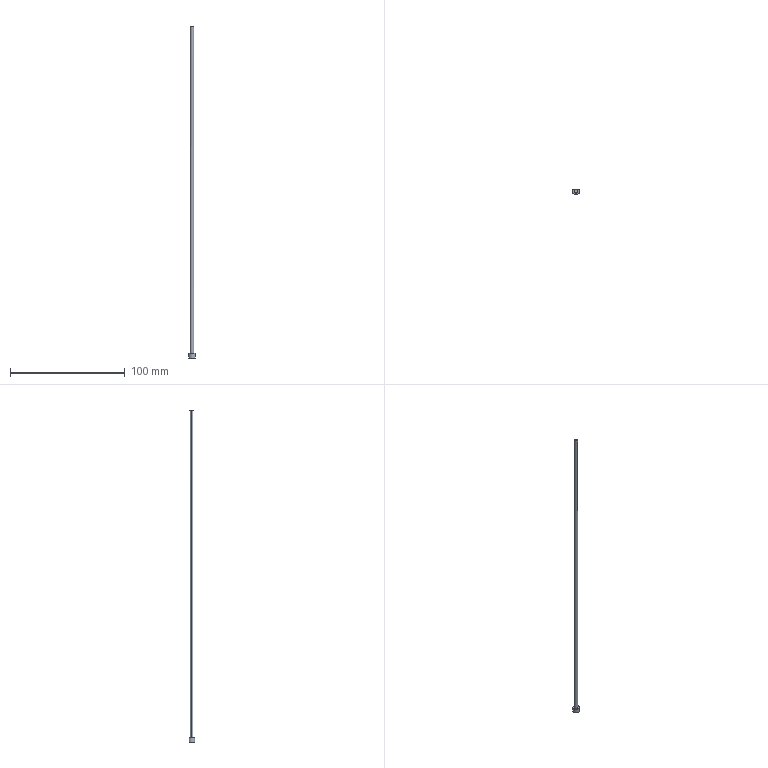Part | Creo | 1 solid | 7 faces | box 6 x 5 x 289.623 mm | volume 2118 mm3 | plane 4 | cylinder 3 | commonest cylinder face diameters 3 x2 6 x1
STEP:
#1=CARTESIAN_POINT('',(60.264,64.5,-292.));
#2=VERTEX_POINT('',#1);
#3=CARTESIAN_POINT('',(59.5,62.5,-292.));
#4=VERTEX_POINT('',#3);
#5=CARTESIAN_POINT('',(62.5,62.5,-292.));
#6=DIRECTION('',(0.,0.,1.));
#7=DIRECTION('',(-0.7454,0.6667,0.));
#8=AXIS2_PLACEMENT_3D('',#5,#6,#7);
#9=CIRCLE('',#8,3.);
#10=EDGE_CURVE('',#2,#4,#9,.T.);
#11=ORIENTED_EDGE('',*,*,#10,.F.);
#12=CARTESIAN_POINT('',(64.736,64.5,-292.));
#13=VERTEX_POINT('',#12);
#14=CARTESIAN_POINT('',(64.736,64.5,-292.));
#15=DIRECTION('',(-1.,0.,0.));
#16=VECTOR('',#15,4.472);
#17=LINE('',#14,#16);
#18=EDGE_CURVE('',#13,#2,#17,.T.);
#19=ORIENTED_EDGE('',*,*,#18,.F.);
#20=CARTESIAN_POINT('',(62.5,62.5,-292.));
#21=DIRECTION('',(0.,0.,1.));
#22=DIRECTION('',(-1.,0.,0.));
#23=AXIS2_PLACEMENT_3D('',#20,#21,#22);
#24=CIRCLE('',#23,3.);
#25=EDGE_CURVE('',#4,#13,#24,.T.);
#26=ORIENTED_EDGE('',*,*,#25,.F.);
#27=EDGE_LOOP('',(#11,#19,#26));
#28=FACE_OUTER_BOUND('',#27,.F.);
#29=CARTESIAN_POINT('',(64.,62.5,-292.));
#30=VERTEX_POINT('',#29);
#31=CARTESIAN_POINT('',(61.,62.5,-292.));
#32=VERTEX_POINT('',#31);
#33=CARTESIAN_POINT('',(62.5,62.5,-292.));
#34=DIRECTION('',(0.,0.,-1.));
#35=DIRECTION('',(1.,0.,0.));
#36=AXIS2_PLACEMENT_3D('',#33,#34,#35);
#37=CIRCLE('',#36,1.5);
#38=EDGE_CURVE('',#30,#32,#37,.T.);
#39=ORIENTED_EDGE('',*,*,#38,.F.);
#40=CARTESIAN_POINT('',(62.5,62.5,-292.));
#41=DIRECTION('',(0.,0.,-1.));
#42=DIRECTION('',(-1.,0.,0.));
#43=AXIS2_PLACEMENT_3D('',#40,#41,#42);
#44=CIRCLE('',#43,1.5);
#45=EDGE_CURVE('',#32,#30,#44,.T.);
#46=ORIENTED_EDGE('',*,*,#45,.F.);
#47=EDGE_LOOP('',(#39,#46));
#48=FACE_BOUND('',#47,.F.);
#49=CARTESIAN_POINT('',(62.5,62.5,-292.));
#50=DIRECTION('',(0.,0.,1.));
#51=DIRECTION('',(-1.,0.,0.));
#52=AXIS2_PLACEMENT_3D('',#49,#50,#51);
#53=PLANE('',#52);
#54=ADVANCED_FACE('',(#28,#48),#53,.T.);
#55=ORIENTED_EDGE('',*,*,#38,.T.);
#56=CARTESIAN_POINT('',(61.,62.5,-6.377));
#57=VERTEX_POINT('',#56);
#58=CARTESIAN_POINT('',(61.,62.5,-292.));
#59=DIRECTION('',(0.,0.000000001,1.));
#60=VECTOR('',#59,285.623);
#61=LINE('',#58,#60);
#62=EDGE_CURVE('',#32,#57,#61,.T.);
#63=ORIENTED_EDGE('',*,*,#62,.T.);
#64=CARTESIAN_POINT('',(64.,62.5,-6.535));
#65=VERTEX_POINT('',#64);
#66=CARTESIAN_POINT('',(61.,62.5,-6.377));
#67=CARTESIAN_POINT('',(61.,62.146,-6.377));
#68=CARTESIAN_POINT('',(61.223,61.523,-6.389));
#69=CARTESIAN_POINT('',(61.946,61.064,-6.427));
#70=CARTESIAN_POINT('',(62.5,60.968,-6.456));
#71=CARTESIAN_POINT('',(63.054,61.064,-6.485));
#72=CARTESIAN_POINT('',(63.777,61.523,-6.523));
#73=CARTESIAN_POINT('',(64.,62.146,-6.535));
#74=CARTESIAN_POINT('',(64.,62.5,-6.535));
#75=B_SPLINE_CURVE_WITH_KNOTS('',3,(#66,#67,#68,#69,#70,#71,#72,#73,#74),.UNSPECIFIED.,.F.,.F.,(4,1,1,1,1,1,4),(0.,0.25,0.375,0.5,0.625,0.75,1.),.UNSPECIFIED.);
#76=EDGE_CURVE('',#57,#65,#75,.T.);
#77=ORIENTED_EDGE('',*,*,#76,.T.);
#78=CARTESIAN_POINT('',(64.,62.5,-292.));
#79=DIRECTION('',(0.,0.,1.));
#80=VECTOR('',#79,285.465);
#81=LINE('',#78,#80);
#82=EDGE_CURVE('',#30,#65,#81,.T.);
#83=ORIENTED_EDGE('',*,*,#82,.F.);
#84=EDGE_LOOP('',(#55,#63,#77,#83));
#85=FACE_OUTER_BOUND('',#84,.F.);
#86=CARTESIAN_POINT('',(62.5,62.5,-352.221));
#87=DIRECTION('',(0.,0.,1.));
#88=DIRECTION('',(-1.,0.,0.));
#89=AXIS2_PLACEMENT_3D('',#86,#87,#88);
#90=CYLINDRICAL_SURFACE('',#89,1.5);
#91=ADVANCED_FACE('',(#85),#90,.T.);
#92=ORIENTED_EDGE('',*,*,#45,.T.);
#93=ORIENTED_EDGE('',*,*,#82,.T.);
#94=CARTESIAN_POINT('',(64.,62.5,-6.535));
#95=CARTESIAN_POINT('',(64.,62.854,-6.535));
#96=CARTESIAN_POINT('',(63.777,63.477,-6.523));
#97=CARTESIAN_POINT('',(63.054,63.936,-6.485));
#98=CARTESIAN_POINT('',(62.5,64.032,-6.456));
#99=CARTESIAN_POINT('',(61.946,63.936,-6.427));
#100=CARTESIAN_POINT('',(61.223,63.477,-6.389));
#101=CARTESIAN_POINT('',(61.,62.854,-6.377));
#102=CARTESIAN_POINT('',(61.,62.5,-6.377));
#103=B_SPLINE_CURVE_WITH_KNOTS('',3,(#94,#95,#96,#97,#98,#99,#100,#101,#102),.UNSPECIFIED.,.F.,.F.,(4,1,1,1,1,1,4),(0.,0.25,0.375,0.5,0.625,0.75,1.),.UNSPECIFIED.);
#104=EDGE_CURVE('',#65,#57,#103,.T.);
#105=ORIENTED_EDGE('',*,*,#104,.T.);
#106=ORIENTED_EDGE('',*,*,#62,.F.);
#107=EDGE_LOOP('',(#92,#93,#105,#106));
#108=FACE_OUTER_BOUND('',#107,.F.);
#109=CARTESIAN_POINT('',(62.5,62.5,-352.221));
#110=DIRECTION('',(0.,0.,1.));
#111=DIRECTION('',(-1.,0.,0.));
#112=AXIS2_PLACEMENT_3D('',#109,#110,#111);
#113=CYLINDRICAL_SURFACE('',#112,1.5);
#114=ADVANCED_FACE('',(#108),#113,.T.);
#115=ORIENTED_EDGE('',*,*,#76,.F.);
#116=ORIENTED_EDGE('',*,*,#104,.F.);
#117=EDGE_LOOP('',(#115,#116));
#118=FACE_OUTER_BOUND('',#117,.F.);
#119=CARTESIAN_POINT('',(308.361,-226.75,-19.338));
#120=DIRECTION('',(0.05232,-0.000000032,0.9986));
#121=DIRECTION('',(-0.000000001,-1.,-0.000000032));
#122=AXIS2_PLACEMENT_3D('',#119,#120,#121);
#123=PLANE('',#122);
#124=ADVANCED_FACE('',(#118),#123,.T.);
#125=CARTESIAN_POINT('',(60.264,64.5,-296.));
#126=VERTEX_POINT('',#125);
#127=CARTESIAN_POINT('',(60.264,64.5,-292.));
#128=DIRECTION('',(0.,0.,-1.));
#129=VECTOR('',#128,4.);
#130=LINE('',#127,#129);
#131=EDGE_CURVE('',#2,#126,#130,.T.);
#132=ORIENTED_EDGE('',*,*,#131,.F.);
#133=ORIENTED_EDGE('',*,*,#10,.T.);
#134=ORIENTED_EDGE('',*,*,#25,.T.);
#135=CARTESIAN_POINT('',(64.736,64.5,-296.));
#136=VERTEX_POINT('',#135);
#137=CARTESIAN_POINT('',(64.736,64.5,-296.));
#138=DIRECTION('',(0.,0.,1.));
#139=VECTOR('',#138,4.);
#140=LINE('',#137,#139);
#141=EDGE_CURVE('',#136,#13,#140,.T.);
#142=ORIENTED_EDGE('',*,*,#141,.F.);
#143=CARTESIAN_POINT('',(59.5,62.5,-296.));
#144=VERTEX_POINT('',#143);
#145=CARTESIAN_POINT('',(62.5,62.5,-296.));
#146=DIRECTION('',(0.,0.,-1.));
#147=DIRECTION('',(0.7454,0.6667,0.));
#148=AXIS2_PLACEMENT_3D('',#145,#146,#147);
#149=CIRCLE('',#148,3.);
#150=EDGE_CURVE('',#136,#144,#149,.T.);
#151=ORIENTED_EDGE('',*,*,#150,.T.);
#152=CARTESIAN_POINT('',(62.5,62.5,-296.));
#153=DIRECTION('',(0.,0.,-1.));
#154=DIRECTION('',(-1.,0.,0.));
#155=AXIS2_PLACEMENT_3D('',#152,#153,#154);
#156=CIRCLE('',#155,3.);
#157=EDGE_CURVE('',#144,#126,#156,.T.);
#158=ORIENTED_EDGE('',*,*,#157,.T.);
#159=EDGE_LOOP('',(#132,#133,#134,#142,#151,#158));
#160=FACE_OUTER_BOUND('',#159,.F.);
#161=CARTESIAN_POINT('',(62.5,62.5,-296.));
#162=DIRECTION('',(0.,0.,1.));
#163=DIRECTION('',(-1.,0.,0.));
#164=AXIS2_PLACEMENT_3D('',#161,#162,#163);
#165=CYLINDRICAL_SURFACE('',#164,3.);
#166=ADVANCED_FACE('',(#160),#165,.T.);
#167=ORIENTED_EDGE('',*,*,#131,.T.);
#168=CARTESIAN_POINT('',(60.264,64.5,-296.));
#169=DIRECTION('',(1.,0.,0.));
#170=VECTOR('',#169,4.472);
#171=LINE('',#168,#170);
#172=EDGE_CURVE('',#126,#136,#171,.T.);
#173=ORIENTED_EDGE('',*,*,#172,.T.);
#174=ORIENTED_EDGE('',*,*,#141,.T.);
#175=ORIENTED_EDGE('',*,*,#18,.T.);
#176=EDGE_LOOP('',(#167,#173,#174,#175));
#177=FACE_OUTER_BOUND('',#176,.F.);
#178=CARTESIAN_POINT('',(62.5,64.5,-297.8));
#179=DIRECTION('',(0.,-1.,0.));
#180=DIRECTION('',(0.,0.,-1.));
#181=AXIS2_PLACEMENT_3D('',#178,#179,#180);
#182=PLANE('',#181);
#183=ADVANCED_FACE('',(#177),#182,.F.);
#184=ORIENTED_EDGE('',*,*,#150,.F.);
#185=ORIENTED_EDGE('',*,*,#172,.F.);
#186=ORIENTED_EDGE('',*,*,#157,.F.);
#187=EDGE_LOOP('',(#184,#185,#186));
#188=FACE_OUTER_BOUND('',#187,.F.);
#189=CARTESIAN_POINT('',(10.,125.005,-296.));
#190=DIRECTION('',(0.,0.,1.));
#191=DIRECTION('',(0.,-1.,0.));
#192=AXIS2_PLACEMENT_3D('',#189,#190,#191);
#193=PLANE('',#192);
#194=ADVANCED_FACE('',(#188),#193,.F.);
#195=CLOSED_SHELL('',(#54,#91,#114,#124,#166,#183,#194));
#196=MANIFOLD_SOLID_BREP('',#195);
#197=(LENGTH_UNIT()NAMED_UNIT(*)SI_UNIT(.MILLI.,.METRE.));
#198=UNCERTAINTY_MEASURE_WITH_UNIT(LENGTH_MEASURE(0.02897),#197,'','');
#199=(NAMED_UNIT(*)PLANE_ANGLE_UNIT()SI_UNIT($,.RADIAN.));
#200=PLANE_ANGLE_MEASURE_WITH_UNIT(PLANE_ANGLE_MEASURE(0.01745),#199);
#201=(CONVERSION_BASED_UNIT('DEGREE',#200)NAMED_UNIT(*)PLANE_ANGLE_UNIT());
#202=(NAMED_UNIT(*)SI_UNIT($,.STERADIAN.)SOLID_ANGLE_UNIT());
#203=(GEOMETRIC_REPRESENTATION_CONTEXT(3)GLOBAL_UNCERTAINTY_ASSIGNED_CONTEXT((#198))GLOBAL_UNIT_ASSIGNED_CONTEXT((#197,#201,#202))REPRESENTATION_CONTEXT('',''));
#204=ADVANCED_BREP_SHAPE_REPRESENTATION('',(#196),#203);